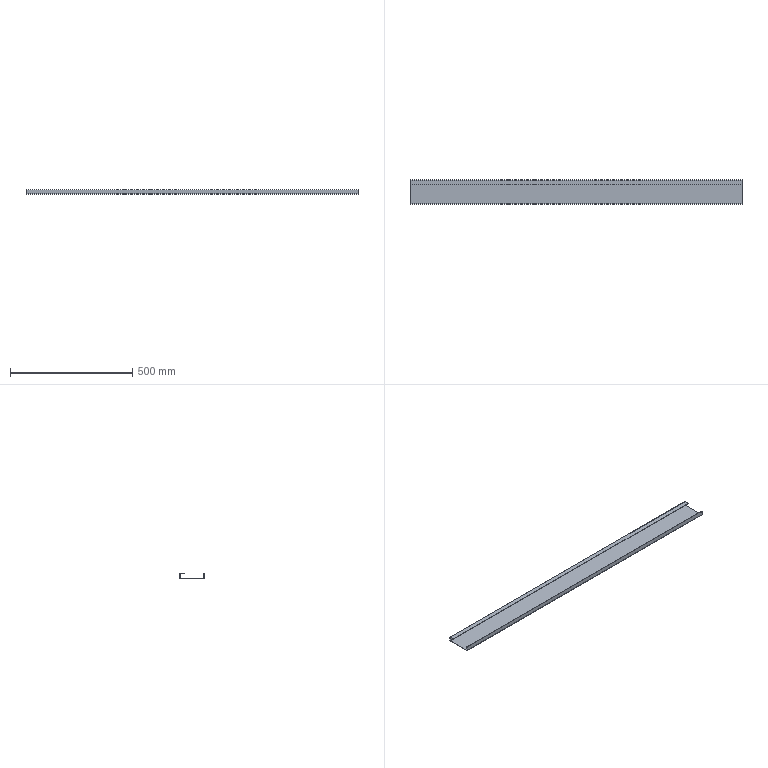Part | STEP file | 电柜护栏3踢脚Plate | 1 solid | 18 faces | box 1360 x 100 x 20 mm | volume 312623 mm3 | plane 12 | cylinder 6 | commonest cylinder face diameters 2 x3 5 x3
STEP:
#1=CARTESIAN_POINT('',(0.,0.,0.));
#2=DIRECTION('',(0.,0.,1.));
#3=DIRECTION('',(1.,0.,0.));
#4=AXIS2_PLACEMENT_3D('',#1,#2,#3);
#5=CARTESIAN_POINT('',(-680.,1.5,2.5));
#6=VERTEX_POINT('',#5);
#7=CARTESIAN_POINT('',(-680.,1.5,20.));
#8=VERTEX_POINT('',#7);
#9=CARTESIAN_POINT('',(-680.,1.5,2.5));
#10=DIRECTION('',(0.,0.,1.));
#11=VECTOR('',#10,1.);
#12=LINE('',#9,#11);
#13=CARTESIAN_POINT('',(680.,1.5,2.5));
#14=DIRECTION('',(0.,-1.,0.));
#15=DIRECTION('',(0.,0.,-1.));
#16=AXIS2_PLACEMENT_3D('',#13,#14,#15);
#17=PLANE('',#16);
#18=CARTESIAN_POINT('',(0.,-1360.));
#19=DIRECTION('',(-1.,0.));
#20=VECTOR('',#19,1.);
#21=LINE('',#18,#20);
#22=(GEOMETRIC_REPRESENTATION_CONTEXT(2)PARAMETRIC_REPRESENTATION_CONTEXT()REPRESENTATION_CONTEXT('',''));
#23=DEFINITIONAL_REPRESENTATION('',(#21),#22);
#24=PCURVE('',#17,#23);
#25=CARTESIAN_POINT('',(-680.,2.5,2.5));
#26=DIRECTION('',(-1.,0.,0.));
#27=DIRECTION('',(0.,0.,1.));
#28=AXIS2_PLACEMENT_3D('',#25,#26,#27);
#29=PLANE('',#28);
#30=CARTESIAN_POINT('',(0.,-1.));
#31=DIRECTION('',(1.,0.));
#32=VECTOR('',#31,1.);
#33=LINE('',#30,#32);
#34=(GEOMETRIC_REPRESENTATION_CONTEXT(2)PARAMETRIC_REPRESENTATION_CONTEXT()REPRESENTATION_CONTEXT('',''));
#35=DEFINITIONAL_REPRESENTATION('',(#33),#34);
#36=PCURVE('',#29,#35);
#37=SURFACE_CURVE('',#12,(#24,#36),.PCURVE_S1.);
#38=EDGE_CURVE('',#6,#8,#37,.T.);
#39=ORIENTED_EDGE('',*,*,#38,.T.);
#40=CARTESIAN_POINT('',(680.,1.5,20.));
#41=VERTEX_POINT('',#40);
#42=CARTESIAN_POINT('',(680.,1.5,20.));
#43=DIRECTION('',(-1.,0.,0.));
#44=VECTOR('',#43,1.);
#45=LINE('',#42,#44);
#46=CARTESIAN_POINT('',(-17.5,0.));
#47=DIRECTION('',(0.,-1.));
#48=VECTOR('',#47,1.);
#49=LINE('',#46,#48);
#50=(GEOMETRIC_REPRESENTATION_CONTEXT(2)PARAMETRIC_REPRESENTATION_CONTEXT()REPRESENTATION_CONTEXT('',''));
#51=DEFINITIONAL_REPRESENTATION('',(#49),#50);
#52=PCURVE('',#17,#51);
#53=CARTESIAN_POINT('',(680.,0.,20.));
#54=DIRECTION('',(0.,0.,1.));
#55=DIRECTION('',(1.,0.,0.));
#56=AXIS2_PLACEMENT_3D('',#53,#54,#55);
#57=PLANE('',#56);
#58=CARTESIAN_POINT('',(0.,1.5));
#59=DIRECTION('',(-1.,0.));
#60=VECTOR('',#59,1.);
#61=LINE('',#58,#60);
#62=(GEOMETRIC_REPRESENTATION_CONTEXT(2)PARAMETRIC_REPRESENTATION_CONTEXT()REPRESENTATION_CONTEXT('',''));
#63=DEFINITIONAL_REPRESENTATION('',(#61),#62);
#64=PCURVE('',#57,#63);
#65=SURFACE_CURVE('',#45,(#52,#64),.PCURVE_S1.);
#66=EDGE_CURVE('',#41,#8,#65,.T.);
#67=ORIENTED_EDGE('',*,*,#66,.F.);
#68=CARTESIAN_POINT('',(680.,1.5,2.5));
#69=VERTEX_POINT('',#68);
#70=CARTESIAN_POINT('',(680.,1.5,2.5));
#71=DIRECTION('',(0.,0.,1.));
#72=VECTOR('',#71,1.);
#73=LINE('',#70,#72);
#74=CARTESIAN_POINT('',(0.,0.));
#75=DIRECTION('',(-1.,0.));
#76=VECTOR('',#75,1.);
#77=LINE('',#74,#76);
#78=(GEOMETRIC_REPRESENTATION_CONTEXT(2)PARAMETRIC_REPRESENTATION_CONTEXT()REPRESENTATION_CONTEXT('',''));
#79=DEFINITIONAL_REPRESENTATION('',(#77),#78);
#80=PCURVE('',#17,#79);
#81=CARTESIAN_POINT('',(680.,2.5,2.5));
#82=DIRECTION('',(-1.,0.,0.));
#83=DIRECTION('',(0.,0.,1.));
#84=AXIS2_PLACEMENT_3D('',#81,#82,#83);
#85=PLANE('',#84);
#86=CARTESIAN_POINT('',(0.,-1.));
#87=DIRECTION('',(1.,0.));
#88=VECTOR('',#87,1.);
#89=LINE('',#86,#88);
#90=(GEOMETRIC_REPRESENTATION_CONTEXT(2)PARAMETRIC_REPRESENTATION_CONTEXT()REPRESENTATION_CONTEXT('',''));
#91=DEFINITIONAL_REPRESENTATION('',(#89),#90);
#92=PCURVE('',#85,#91);
#93=SURFACE_CURVE('',#73,(#80,#92),.PCURVE_S1.);
#94=EDGE_CURVE('',#69,#41,#93,.T.);
#95=ORIENTED_EDGE('',*,*,#94,.F.);
#96=CARTESIAN_POINT('',(680.,1.5,2.5));
#97=DIRECTION('',(-1.,0.,0.));
#98=VECTOR('',#97,1.);
#99=LINE('',#96,#98);
#100=CARTESIAN_POINT('',(0.,0.));
#101=DIRECTION('',(0.,-1.));
#102=VECTOR('',#101,1.);
#103=LINE('',#100,#102);
#104=(GEOMETRIC_REPRESENTATION_CONTEXT(2)PARAMETRIC_REPRESENTATION_CONTEXT()REPRESENTATION_CONTEXT('',''));
#105=DEFINITIONAL_REPRESENTATION('',(#103),#104);
#106=PCURVE('',#17,#105);
#107=CARTESIAN_POINT('',(680.,2.5,2.5));
#108=DIRECTION('',(-1.,0.,0.));
#109=DIRECTION('',(0.,0.,1.));
#110=AXIS2_PLACEMENT_3D('',#107,#108,#109);
#111=CYLINDRICAL_SURFACE('',#110,1.);
#112=CARTESIAN_POINT('',(4.712,0.));
#113=DIRECTION('',(0.,1.));
#114=VECTOR('',#113,1.);
#115=LINE('',#112,#114);
#116=(GEOMETRIC_REPRESENTATION_CONTEXT(2)PARAMETRIC_REPRESENTATION_CONTEXT()REPRESENTATION_CONTEXT('',''));
#117=DEFINITIONAL_REPRESENTATION('',(#115),#116);
#118=PCURVE('',#111,#117);
#119=SURFACE_CURVE('',#99,(#106,#118),.PCURVE_S1.);
#120=EDGE_CURVE('',#69,#6,#119,.T.);
#121=ORIENTED_EDGE('',*,*,#120,.T.);
#122=EDGE_LOOP('',(#39,#67,#95,#121));
#123=FACE_BOUND('',#122,.T.);
#124=ADVANCED_FACE('',(#123),#17,.F.);
#125=CARTESIAN_POINT('',(-680.,0.,20.));
#126=VERTEX_POINT('',#125);
#127=CARTESIAN_POINT('',(-680.,0.,20.));
#128=DIRECTION('',(0.,1.,0.));
#129=VECTOR('',#128,1.);
#130=LINE('',#127,#129);
#131=CARTESIAN_POINT('',(-1360.,0.));
#132=DIRECTION('',(0.,1.));
#133=VECTOR('',#132,1.);
#134=LINE('',#131,#133);
#135=(GEOMETRIC_REPRESENTATION_CONTEXT(2)PARAMETRIC_REPRESENTATION_CONTEXT()REPRESENTATION_CONTEXT('',''));
#136=DEFINITIONAL_REPRESENTATION('',(#134),#135);
#137=PCURVE('',#57,#136);
#138=CARTESIAN_POINT('',(17.5,-2.5));
#139=DIRECTION('',(0.,1.));
#140=VECTOR('',#139,1.);
#141=LINE('',#138,#140);
#142=(GEOMETRIC_REPRESENTATION_CONTEXT(2)PARAMETRIC_REPRESENTATION_CONTEXT()REPRESENTATION_CONTEXT('',''));
#143=DEFINITIONAL_REPRESENTATION('',(#141),#142);
#144=PCURVE('',#29,#143);
#145=SURFACE_CURVE('',#130,(#137,#144),.PCURVE_S1.);
#146=EDGE_CURVE('',#126,#8,#145,.T.);
#147=ORIENTED_EDGE('',*,*,#146,.F.);
#148=CARTESIAN_POINT('',(680.,0.,20.));
#149=VERTEX_POINT('',#148);
#150=CARTESIAN_POINT('',(680.,0.,20.));
#151=DIRECTION('',(-1.,0.,0.));
#152=VECTOR('',#151,1.);
#153=LINE('',#150,#152);
#154=CARTESIAN_POINT('',(0.,0.));
#155=DIRECTION('',(-1.,0.));
#156=VECTOR('',#155,1.);
#157=LINE('',#154,#156);
#158=(GEOMETRIC_REPRESENTATION_CONTEXT(2)PARAMETRIC_REPRESENTATION_CONTEXT()REPRESENTATION_CONTEXT('',''));
#159=DEFINITIONAL_REPRESENTATION('',(#157),#158);
#160=PCURVE('',#57,#159);
#161=CARTESIAN_POINT('',(680.,0.,2.5));
#162=DIRECTION('',(0.,-1.,0.));
#163=DIRECTION('',(0.,0.,-1.));
#164=AXIS2_PLACEMENT_3D('',#161,#162,#163);
#165=PLANE('',#164);
#166=CARTESIAN_POINT('',(-17.5,0.));
#167=DIRECTION('',(0.,-1.));
#168=VECTOR('',#167,1.);
#169=LINE('',#166,#168);
#170=(GEOMETRIC_REPRESENTATION_CONTEXT(2)PARAMETRIC_REPRESENTATION_CONTEXT()REPRESENTATION_CONTEXT('',''));
#171=DEFINITIONAL_REPRESENTATION('',(#169),#170);
#172=PCURVE('',#165,#171);
#173=SURFACE_CURVE('',#153,(#160,#172),.PCURVE_S1.);
#174=EDGE_CURVE('',#149,#126,#173,.T.);
#175=ORIENTED_EDGE('',*,*,#174,.F.);
#176=CARTESIAN_POINT('',(680.,0.,20.));
#177=DIRECTION('',(0.,1.,0.));
#178=VECTOR('',#177,1.);
#179=LINE('',#176,#178);
#180=CARTESIAN_POINT('',(0.,0.));
#181=DIRECTION('',(0.,1.));
#182=VECTOR('',#181,1.);
#183=LINE('',#180,#182);
#184=(GEOMETRIC_REPRESENTATION_CONTEXT(2)PARAMETRIC_REPRESENTATION_CONTEXT()REPRESENTATION_CONTEXT('',''));
#185=DEFINITIONAL_REPRESENTATION('',(#183),#184);
#186=PCURVE('',#57,#185);
#187=CARTESIAN_POINT('',(17.5,-2.5));
#188=DIRECTION('',(0.,1.));
#189=VECTOR('',#188,1.);
#190=LINE('',#187,#189);
#191=(GEOMETRIC_REPRESENTATION_CONTEXT(2)PARAMETRIC_REPRESENTATION_CONTEXT()REPRESENTATION_CONTEXT('',''));
#192=DEFINITIONAL_REPRESENTATION('',(#190),#191);
#193=PCURVE('',#85,#192);
#194=SURFACE_CURVE('',#179,(#186,#193),.PCURVE_S1.);
#195=EDGE_CURVE('',#149,#41,#194,.T.);
#196=ORIENTED_EDGE('',*,*,#195,.T.);
#197=ORIENTED_EDGE('',*,*,#66,.T.);
#198=EDGE_LOOP('',(#147,#175,#196,#197));
#199=FACE_BOUND('',#198,.T.);
#200=ADVANCED_FACE('',(#199),#57,.T.);
#201=CARTESIAN_POINT('',(-680.,0.,2.5));
#202=VERTEX_POINT('',#201);
#203=CARTESIAN_POINT('',(-680.,0.,2.5));
#204=DIRECTION('',(0.,0.,1.));
#205=VECTOR('',#204,1.);
#206=LINE('',#203,#205);
#207=CARTESIAN_POINT('',(0.,-1360.));
#208=DIRECTION('',(-1.,0.));
#209=VECTOR('',#208,1.);
#210=LINE('',#207,#209);
#211=(GEOMETRIC_REPRESENTATION_CONTEXT(2)PARAMETRIC_REPRESENTATION_CONTEXT()REPRESENTATION_CONTEXT('',''));
#212=DEFINITIONAL_REPRESENTATION('',(#210),#211);
#213=PCURVE('',#165,#212);
#214=CARTESIAN_POINT('',(0.,-2.5));
#215=DIRECTION('',(1.,0.));
#216=VECTOR('',#215,1.);
#217=LINE('',#214,#216);
#218=(GEOMETRIC_REPRESENTATION_CONTEXT(2)PARAMETRIC_REPRESENTATION_CONTEXT()REPRESENTATION_CONTEXT('',''));
#219=DEFINITIONAL_REPRESENTATION('',(#217),#218);
#220=PCURVE('',#29,#219);
#221=SURFACE_CURVE('',#206,(#213,#220),.PCURVE_S1.);
#222=EDGE_CURVE('',#202,#126,#221,.T.);
#223=ORIENTED_EDGE('',*,*,#222,.F.);
#224=CARTESIAN_POINT('',(680.,0.,2.5));
#225=VERTEX_POINT('',#224);
#226=CARTESIAN_POINT('',(680.,0.,2.5));
#227=DIRECTION('',(-1.,0.,0.));
#228=VECTOR('',#227,1.);
#229=LINE('',#226,#228);
#230=CARTESIAN_POINT('',(0.,0.));
#231=DIRECTION('',(0.,-1.));
#232=VECTOR('',#231,1.);
#233=LINE('',#230,#232);
#234=(GEOMETRIC_REPRESENTATION_CONTEXT(2)PARAMETRIC_REPRESENTATION_CONTEXT()REPRESENTATION_CONTEXT('',''));
#235=DEFINITIONAL_REPRESENTATION('',(#233),#234);
#236=PCURVE('',#165,#235);
#237=CARTESIAN_POINT('',(680.,2.5,2.5));
#238=DIRECTION('',(-1.,0.,0.));
#239=DIRECTION('',(0.,0.,1.));
#240=AXIS2_PLACEMENT_3D('',#237,#238,#239);
#241=CYLINDRICAL_SURFACE('',#240,2.5);
#242=CARTESIAN_POINT('',(4.712,0.));
#243=DIRECTION('',(0.,1.));
#244=VECTOR('',#243,1.);
#245=LINE('',#242,#244);
#246=(GEOMETRIC_REPRESENTATION_CONTEXT(2)PARAMETRIC_REPRESENTATION_CONTEXT()REPRESENTATION_CONTEXT('',''));
#247=DEFINITIONAL_REPRESENTATION('',(#245),#246);
#248=PCURVE('',#241,#247);
#249=SURFACE_CURVE('',#229,(#236,#248),.PCURVE_S1.);
#250=EDGE_CURVE('',#225,#202,#249,.T.);
#251=ORIENTED_EDGE('',*,*,#250,.F.);
#252=CARTESIAN_POINT('',(680.,0.,2.5));
#253=DIRECTION('',(0.,0.,1.));
#254=VECTOR('',#253,1.);
#255=LINE('',#252,#254);
#256=CARTESIAN_POINT('',(0.,0.));
#257=DIRECTION('',(-1.,0.));
#258=VECTOR('',#257,1.);
#259=LINE('',#256,#258);
#260=(GEOMETRIC_REPRESENTATION_CONTEXT(2)PARAMETRIC_REPRESENTATION_CONTEXT()REPRESENTATION_CONTEXT('',''));
#261=DEFINITIONAL_REPRESENTATION('',(#259),#260);
#262=PCURVE('',#165,#261);
#263=CARTESIAN_POINT('',(0.,-2.5));
#264=DIRECTION('',(1.,0.));
#265=VECTOR('',#264,1.);
#266=LINE('',#263,#265);
#267=(GEOMETRIC_REPRESENTATION_CONTEXT(2)PARAMETRIC_REPRESENTATION_CONTEXT()REPRESENTATION_CONTEXT('',''));
#268=DEFINITIONAL_REPRESENTATION('',(#266),#267);
#269=PCURVE('',#85,#268);
#270=SURFACE_CURVE('',#255,(#262,#269),.PCURVE_S1.);
#271=EDGE_CURVE('',#225,#149,#270,.T.);
#272=ORIENTED_EDGE('',*,*,#271,.T.);
#273=ORIENTED_EDGE('',*,*,#174,.T.);
#274=EDGE_LOOP('',(#223,#251,#272,#273));
#275=FACE_BOUND('',#274,.T.);
#276=ADVANCED_FACE('',(#275),#165,.T.);
#277=CARTESIAN_POINT('',(-680.,2.5,0.));
#278=VERTEX_POINT('',#277);
#279=CARTESIAN_POINT('',(-680.,2.5,2.5));
#280=DIRECTION('',(-1.,0.,0.));
#281=DIRECTION('',(0.,0.,1.));
#282=AXIS2_PLACEMENT_3D('',#279,#280,#281);
#283=CIRCLE('',#282,2.5);
#284=CARTESIAN_POINT('',(0.,1360.));
#285=DIRECTION('',(1.,0.));
#286=VECTOR('',#285,1.);
#287=LINE('',#284,#286);
#288=(GEOMETRIC_REPRESENTATION_CONTEXT(2)PARAMETRIC_REPRESENTATION_CONTEXT()REPRESENTATION_CONTEXT('',''));
#289=DEFINITIONAL_REPRESENTATION('',(#287),#288);
#290=PCURVE('',#241,#289);
#291=CARTESIAN_POINT('',(0.,0.));
#292=DIRECTION('',(1.,0.));
#293=AXIS2_PLACEMENT_2D('',#291,#292);
#294=CIRCLE('',#293,2.5);
#295=(GEOMETRIC_REPRESENTATION_CONTEXT(2)PARAMETRIC_REPRESENTATION_CONTEXT()REPRESENTATION_CONTEXT('',''));
#296=DEFINITIONAL_REPRESENTATION('',(#294),#295);
#297=PCURVE('',#29,#296);
#298=SURFACE_CURVE('',#283,(#290,#297),.PCURVE_S1.);
#299=EDGE_CURVE('',#278,#202,#298,.T.);
#300=ORIENTED_EDGE('',*,*,#299,.F.);
#301=CARTESIAN_POINT('',(680.,2.5,0.));
#302=VERTEX_POINT('',#301);
#303=CARTESIAN_POINT('',(680.,2.5,0.));
#304=DIRECTION('',(-1.,0.,0.));
#305=VECTOR('',#304,1.);
#306=LINE('',#303,#305);
#307=CARTESIAN_POINT('',(3.142,0.));
#308=DIRECTION('',(0.,1.));
#309=VECTOR('',#308,1.);
#310=LINE('',#307,#309);
#311=(GEOMETRIC_REPRESENTATION_CONTEXT(2)PARAMETRIC_REPRESENTATION_CONTEXT()REPRESENTATION_CONTEXT('',''));
#312=DEFINITIONAL_REPRESENTATION('',(#310),#311);
#313=PCURVE('',#241,#312);
#314=CARTESIAN_POINT('',(680.,2.5,0.));
#315=DIRECTION('',(0.,0.,-1.));
#316=DIRECTION('',(-1.,0.,0.));
#317=AXIS2_PLACEMENT_3D('',#314,#315,#316);
#318=PLANE('',#317);
#319=CARTESIAN_POINT('',(0.,0.));
#320=DIRECTION('',(1.,0.));
#321=VECTOR('',#320,1.);
#322=LINE('',#319,#321);
#323=(GEOMETRIC_REPRESENTATION_CONTEXT(2)PARAMETRIC_REPRESENTATION_CONTEXT()REPRESENTATION_CONTEXT('',''));
#324=DEFINITIONAL_REPRESENTATION('',(#322),#323);
#325=PCURVE('',#318,#324);
#326=SURFACE_CURVE('',#306,(#313,#325),.PCURVE_S1.);
#327=EDGE_CURVE('',#302,#278,#326,.T.);
#328=ORIENTED_EDGE('',*,*,#327,.F.);
#329=CARTESIAN_POINT('',(680.,2.5,2.5));
#330=DIRECTION('',(-1.,0.,0.));
#331=DIRECTION('',(0.,0.,1.));
#332=AXIS2_PLACEMENT_3D('',#329,#330,#331);
#333=CIRCLE('',#332,2.5);
#334=CARTESIAN_POINT('',(0.,0.));
#335=DIRECTION('',(1.,0.));
#336=VECTOR('',#335,1.);
#337=LINE('',#334,#336);
#338=(GEOMETRIC_REPRESENTATION_CONTEXT(2)PARAMETRIC_REPRESENTATION_CONTEXT()REPRESENTATION_CONTEXT('',''));
#339=DEFINITIONAL_REPRESENTATION('',(#337),#338);
#340=PCURVE('',#241,#339);
#341=CARTESIAN_POINT('',(0.,0.));
#342=DIRECTION('',(1.,0.));
#343=AXIS2_PLACEMENT_2D('',#341,#342);
#344=CIRCLE('',#343,2.5);
#345=(GEOMETRIC_REPRESENTATION_CONTEXT(2)PARAMETRIC_REPRESENTATION_CONTEXT()REPRESENTATION_CONTEXT('',''));
#346=DEFINITIONAL_REPRESENTATION('',(#344),#345);
#347=PCURVE('',#85,#346);
#348=SURFACE_CURVE('',#333,(#340,#347),.PCURVE_S1.);
#349=EDGE_CURVE('',#302,#225,#348,.T.);
#350=ORIENTED_EDGE('',*,*,#349,.T.);
#351=ORIENTED_EDGE('',*,*,#250,.T.);
#352=EDGE_LOOP('',(#300,#328,#350,#351));
#353=FACE_BOUND('',#352,.T.);
#354=ADVANCED_FACE('',(#353),#241,.T.);
#355=CARTESIAN_POINT('',(-680.,97.5,0.));
#356=VERTEX_POINT('',#355);
#357=CARTESIAN_POINT('',(-680.,2.5,0.));
#358=DIRECTION('',(0.,-1.,0.));
#359=VECTOR('',#358,1.);
#360=LINE('',#357,#359);
#361=CARTESIAN_POINT('',(1360.,0.));
#362=DIRECTION('',(0.,-1.));
#363=VECTOR('',#362,1.);
#364=LINE('',#361,#363);
#365=(GEOMETRIC_REPRESENTATION_CONTEXT(2)PARAMETRIC_REPRESENTATION_CONTEXT()REPRESENTATION_CONTEXT('',''));
#366=DEFINITIONAL_REPRESENTATION('',(#364),#365);
#367=PCURVE('',#318,#366);
#368=CARTESIAN_POINT('',(-2.5,0.));
#369=DIRECTION('',(0.,-1.));
#370=VECTOR('',#369,1.);
#371=LINE('',#368,#370);
#372=(GEOMETRIC_REPRESENTATION_CONTEXT(2)PARAMETRIC_REPRESENTATION_CONTEXT()REPRESENTATION_CONTEXT('',''));
#373=DEFINITIONAL_REPRESENTATION('',(#371),#372);
#374=PCURVE('',#29,#373);
#375=SURFACE_CURVE('',#360,(#367,#374),.PCURVE_S1.);
#376=EDGE_CURVE('',#356,#278,#375,.T.);
#377=ORIENTED_EDGE('',*,*,#376,.F.);
#378=CARTESIAN_POINT('',(680.,97.5,0.));
#379=VERTEX_POINT('',#378);
#380=CARTESIAN_POINT('',(680.,97.5,0.));
#381=DIRECTION('',(-1.,0.,0.));
#382=VECTOR('',#381,1.);
#383=LINE('',#380,#382);
#384=CARTESIAN_POINT('',(0.,95.));
#385=DIRECTION('',(1.,0.));
#386=VECTOR('',#385,1.);
#387=LINE('',#384,#386);
#388=(GEOMETRIC_REPRESENTATION_CONTEXT(2)PARAMETRIC_REPRESENTATION_CONTEXT()REPRESENTATION_CONTEXT('',''));
#389=DEFINITIONAL_REPRESENTATION('',(#387),#388);
#390=PCURVE('',#318,#389);
#391=CARTESIAN_POINT('',(680.,97.5,2.5));
#392=DIRECTION('',(-1.,0.,0.));
#393=DIRECTION('',(0.,0.,1.));
#394=AXIS2_PLACEMENT_3D('',#391,#392,#393);
#395=CYLINDRICAL_SURFACE('',#394,2.5);
#396=CARTESIAN_POINT('',(3.142,0.));
#397=DIRECTION('',(0.,1.));
#398=VECTOR('',#397,1.);
#399=LINE('',#396,#398);
#400=(GEOMETRIC_REPRESENTATION_CONTEXT(2)PARAMETRIC_REPRESENTATION_CONTEXT()REPRESENTATION_CONTEXT('',''));
#401=DEFINITIONAL_REPRESENTATION('',(#399),#400);
#402=PCURVE('',#395,#401);
#403=SURFACE_CURVE('',#383,(#390,#402),.PCURVE_S1.);
#404=EDGE_CURVE('',#379,#356,#403,.T.);
#405=ORIENTED_EDGE('',*,*,#404,.F.);
#406=CARTESIAN_POINT('',(680.,2.5,0.));
#407=DIRECTION('',(0.,-1.,0.));
#408=VECTOR('',#407,1.);
#409=LINE('',#406,#408);
#410=CARTESIAN_POINT('',(0.,0.));
#411=DIRECTION('',(0.,-1.));
#412=VECTOR('',#411,1.);
#413=LINE('',#410,#412);
#414=(GEOMETRIC_REPRESENTATION_CONTEXT(2)PARAMETRIC_REPRESENTATION_CONTEXT()REPRESENTATION_CONTEXT('',''));
#415=DEFINITIONAL_REPRESENTATION('',(#413),#414);
#416=PCURVE('',#318,#415);
#417=CARTESIAN_POINT('',(-2.5,0.));
#418=DIRECTION('',(0.,-1.));
#419=VECTOR('',#418,1.);
#420=LINE('',#417,#419);
#421=(GEOMETRIC_REPRESENTATION_CONTEXT(2)PARAMETRIC_REPRESENTATION_CONTEXT()REPRESENTATION_CONTEXT('',''));
#422=DEFINITIONAL_REPRESENTATION('',(#420),#421);
#423=PCURVE('',#85,#422);
#424=SURFACE_CURVE('',#409,(#416,#423),.PCURVE_S1.);
#425=EDGE_CURVE('',#379,#302,#424,.T.);
#426=ORIENTED_EDGE('',*,*,#425,.T.);
#427=ORIENTED_EDGE('',*,*,#327,.T.);
#428=EDGE_LOOP('',(#377,#405,#426,#427));
#429=FACE_BOUND('',#428,.T.);
#430=ADVANCED_FACE('',(#429),#318,.T.);
#431=CARTESIAN_POINT('',(-680.,100.,2.5));
#432=VERTEX_POINT('',#431);
#433=CARTESIAN_POINT('',(-680.,97.5,2.5));
#434=DIRECTION('',(-1.,0.,0.));
#435=DIRECTION('',(0.,0.,-1.));
#436=AXIS2_PLACEMENT_3D('',#433,#434,#435);
#437=CIRCLE('',#436,2.5);
#438=CARTESIAN_POINT('',(-3.142,1360.));
#439=DIRECTION('',(1.,0.));
#440=VECTOR('',#439,1.);
#441=LINE('',#438,#440);
#442=(GEOMETRIC_REPRESENTATION_CONTEXT(2)PARAMETRIC_REPRESENTATION_CONTEXT()REPRESENTATION_CONTEXT('',''));
#443=DEFINITIONAL_REPRESENTATION('',(#441),#442);
#444=PCURVE('',#395,#443);
#445=CARTESIAN_POINT('',(0.,95.));
#446=DIRECTION('',(-1.,0.));
#447=AXIS2_PLACEMENT_2D('',#445,#446);
#448=CIRCLE('',#447,2.5);
#449=(GEOMETRIC_REPRESENTATION_CONTEXT(2)PARAMETRIC_REPRESENTATION_CONTEXT()REPRESENTATION_CONTEXT('',''));
#450=DEFINITIONAL_REPRESENTATION('',(#448),#449);
#451=PCURVE('',#29,#450);
#452=SURFACE_CURVE('',#437,(#444,#451),.PCURVE_S1.);
#453=EDGE_CURVE('',#432,#356,#452,.T.);
#454=ORIENTED_EDGE('',*,*,#453,.F.);
#455=CARTESIAN_POINT('',(680.,100.,2.5));
#456=VERTEX_POINT('',#455);
#457=CARTESIAN_POINT('',(680.,100.,2.5));
#458=DIRECTION('',(-1.,0.,0.));
#459=VECTOR('',#458,1.);
#460=LINE('',#457,#459);
#461=CARTESIAN_POINT('',(1.571,0.));
#462=DIRECTION('',(0.,1.));
#463=VECTOR('',#462,1.);
#464=LINE('',#461,#463);
#465=(GEOMETRIC_REPRESENTATION_CONTEXT(2)PARAMETRIC_REPRESENTATION_CONTEXT()REPRESENTATION_CONTEXT('',''));
#466=DEFINITIONAL_REPRESENTATION('',(#464),#465);
#467=PCURVE('',#395,#466);
#468=CARTESIAN_POINT('',(680.,100.,2.5));
#469=DIRECTION('',(0.,1.,0.));
#470=DIRECTION('',(0.,0.,1.));
#471=AXIS2_PLACEMENT_3D('',#468,#469,#470);
#472=PLANE('',#471);
#473=CARTESIAN_POINT('',(0.,0.));
#474=DIRECTION('',(0.,-1.));
#475=VECTOR('',#474,1.);
#476=LINE('',#473,#475);
#477=(GEOMETRIC_REPRESENTATION_CONTEXT(2)PARAMETRIC_REPRESENTATION_CONTEXT()REPRESENTATION_CONTEXT('',''));
#478=DEFINITIONAL_REPRESENTATION('',(#476),#477);
#479=PCURVE('',#472,#478);
#480=SURFACE_CURVE('',#460,(#467,#479),.PCURVE_S1.);
#481=EDGE_CURVE('',#456,#432,#480,.T.);
#482=ORIENTED_EDGE('',*,*,#481,.F.);
#483=CARTESIAN_POINT('',(680.,97.5,2.5));
#484=DIRECTION('',(-1.,0.,0.));
#485=DIRECTION('',(0.,0.,-1.));
#486=AXIS2_PLACEMENT_3D('',#483,#484,#485);
#487=CIRCLE('',#486,2.5);
#488=CARTESIAN_POINT('',(-3.142,0.));
#489=DIRECTION('',(1.,0.));
#490=VECTOR('',#489,1.);
#491=LINE('',#488,#490);
#492=(GEOMETRIC_REPRESENTATION_CONTEXT(2)PARAMETRIC_REPRESENTATION_CONTEXT()REPRESENTATION_CONTEXT('',''));
#493=DEFINITIONAL_REPRESENTATION('',(#491),#492);
#494=PCURVE('',#395,#493);
#495=CARTESIAN_POINT('',(0.,95.));
#496=DIRECTION('',(-1.,0.));
#497=AXIS2_PLACEMENT_2D('',#495,#496);
#498=CIRCLE('',#497,2.5);
#499=(GEOMETRIC_REPRESENTATION_CONTEXT(2)PARAMETRIC_REPRESENTATION_CONTEXT()REPRESENTATION_CONTEXT('',''));
#500=DEFINITIONAL_REPRESENTATION('',(#498),#499);
#501=PCURVE('',#85,#500);
#502=SURFACE_CURVE('',#487,(#494,#501),.PCURVE_S1.);
#503=EDGE_CURVE('',#456,#379,#502,.T.);
#504=ORIENTED_EDGE('',*,*,#503,.T.);
#505=ORIENTED_EDGE('',*,*,#404,.T.);
#506=EDGE_LOOP('',(#454,#482,#504,#505));
#507=FACE_BOUND('',#506,.T.);
#508=ADVANCED_FACE('',(#507),#395,.T.);
#509=CARTESIAN_POINT('',(-680.,100.,17.5));
#510=VERTEX_POINT('',#509);
#511=CARTESIAN_POINT('',(-680.,100.,2.5));
#512=DIRECTION('',(0.,0.,-1.));
#513=VECTOR('',#512,1.);
#514=LINE('',#511,#513);
#515=CARTESIAN_POINT('',(0.,-1360.));
#516=DIRECTION('',(-1.,0.));
#517=VECTOR('',#516,1.);
#518=LINE('',#515,#517);
#519=(GEOMETRIC_REPRESENTATION_CONTEXT(2)PARAMETRIC_REPRESENTATION_CONTEXT()REPRESENTATION_CONTEXT('',''));
#520=DEFINITIONAL_REPRESENTATION('',(#518),#519);
#521=PCURVE('',#472,#520);
#522=CARTESIAN_POINT('',(0.,97.5));
#523=DIRECTION('',(-1.,0.));
#524=VECTOR('',#523,1.);
#525=LINE('',#522,#524);
#526=(GEOMETRIC_REPRESENTATION_CONTEXT(2)PARAMETRIC_REPRESENTATION_CONTEXT()REPRESENTATION_CONTEXT('',''));
#527=DEFINITIONAL_REPRESENTATION('',(#525),#526);
#528=PCURVE('',#29,#527);
#529=SURFACE_CURVE('',#514,(#521,#528),.PCURVE_S1.);
#530=EDGE_CURVE('',#510,#432,#529,.T.);
#531=ORIENTED_EDGE('',*,*,#530,.F.);
#532=CARTESIAN_POINT('',(680.,100.,17.5));
#533=VERTEX_POINT('',#532);
#534=CARTESIAN_POINT('',(680.,100.,17.5));
#535=DIRECTION('',(-1.,0.,0.));
#536=VECTOR('',#535,1.);
#537=LINE('',#534,#536);
#538=CARTESIAN_POINT('',(15.,0.));
#539=DIRECTION('',(0.,-1.));
#540=VECTOR('',#539,1.);
#541=LINE('',#538,#540);
#542=(GEOMETRIC_REPRESENTATION_CONTEXT(2)PARAMETRIC_REPRESENTATION_CONTEXT()REPRESENTATION_CONTEXT('',''));
#543=DEFINITIONAL_REPRESENTATION('',(#541),#542);
#544=PCURVE('',#472,#543);
#545=CARTESIAN_POINT('',(680.,97.5,17.5));
#546=DIRECTION('',(-1.,0.,0.));
#547=DIRECTION('',(0.,0.,1.));
#548=AXIS2_PLACEMENT_3D('',#545,#546,#547);
#549=CYLINDRICAL_SURFACE('',#548,2.5);
#550=CARTESIAN_POINT('',(1.571,0.));
#551=DIRECTION('',(0.,1.));
#552=VECTOR('',#551,1.);
#553=LINE('',#550,#552);
#554=(GEOMETRIC_REPRESENTATION_CONTEXT(2)PARAMETRIC_REPRESENTATION_CONTEXT()REPRESENTATION_CONTEXT('',''));
#555=DEFINITIONAL_REPRESENTATION('',(#553),#554);
#556=PCURVE('',#549,#555);
#557=SURFACE_CURVE('',#537,(#544,#556),.PCURVE_S1.);
#558=EDGE_CURVE('',#533,#510,#557,.T.);
#559=ORIENTED_EDGE('',*,*,#558,.F.);
#560=CARTESIAN_POINT('',(680.,100.,2.5));
#561=DIRECTION('',(0.,0.,-1.));
#562=VECTOR('',#561,1.);
#563=LINE('',#560,#562);
#564=CARTESIAN_POINT('',(0.,0.));
#565=DIRECTION('',(-1.,0.));
#566=VECTOR('',#565,1.);
#567=LINE('',#564,#566);
#568=(GEOMETRIC_REPRESENTATION_CONTEXT(2)PARAMETRIC_REPRESENTATION_CONTEXT()REPRESENTATION_CONTEXT('',''));
#569=DEFINITIONAL_REPRESENTATION('',(#567),#568);
#570=PCURVE('',#472,#569);
#571=CARTESIAN_POINT('',(0.,97.5));
#572=DIRECTION('',(-1.,0.));
#573=VECTOR('',#572,1.);
#574=LINE('',#571,#573);
#575=(GEOMETRIC_REPRESENTATION_CONTEXT(2)PARAMETRIC_REPRESENTATION_CONTEXT()REPRESENTATION_CONTEXT('',''));
#576=DEFINITIONAL_REPRESENTATION('',(#574),#575);
#577=PCURVE('',#85,#576);
#578=SURFACE_CURVE('',#563,(#570,#577),.PCURVE_S1.);
#579=EDGE_CURVE('',#533,#456,#578,.T.);
#580=ORIENTED_EDGE('',*,*,#579,.T.);
#581=ORIENTED_EDGE('',*,*,#481,.T.);
#582=EDGE_LOOP('',(#531,#559,#580,#581));
#583=FACE_BOUND('',#582,.T.);
#584=ADVANCED_FACE('',(#583),#472,.T.);
#585=CARTESIAN_POINT('',(-680.,97.5,20.));
#586=VERTEX_POINT('',#585);
#587=CARTESIAN_POINT('',(-680.,97.5,17.5));
#588=DIRECTION('',(-1.,0.,0.));
#589=DIRECTION('',(0.,0.,-1.));
#590=AXIS2_PLACEMENT_3D('',#587,#588,#589);
#591=CIRCLE('',#590,2.5);
#592=CARTESIAN_POINT('',(-3.142,1360.));
#593=DIRECTION('',(1.,0.));
#594=VECTOR('',#593,1.);
#595=LINE('',#592,#594);
#596=(GEOMETRIC_REPRESENTATION_CONTEXT(2)PARAMETRIC_REPRESENTATION_CONTEXT()REPRESENTATION_CONTEXT('',''));
#597=DEFINITIONAL_REPRESENTATION('',(#595),#596);
#598=PCURVE('',#549,#597);
#599=CARTESIAN_POINT('',(15.,95.));
#600=DIRECTION('',(-1.,0.));
#601=AXIS2_PLACEMENT_2D('',#599,#600);
#602=CIRCLE('',#601,2.5);
#603=(GEOMETRIC_REPRESENTATION_CONTEXT(2)PARAMETRIC_REPRESENTATION_CONTEXT()REPRESENTATION_CONTEXT('',''));
#604=DEFINITIONAL_REPRESENTATION('',(#602),#603);
#605=PCURVE('',#29,#604);
#606=SURFACE_CURVE('',#591,(#598,#605),.PCURVE_S1.);
#607=EDGE_CURVE('',#586,#510,#606,.T.);
#608=ORIENTED_EDGE('',*,*,#607,.F.);
#609=CARTESIAN_POINT('',(680.,97.5,20.));
#610=VERTEX_POINT('',#609);
#611=CARTESIAN_POINT('',(680.,97.5,20.));
#612=DIRECTION('',(-1.,0.,0.));
#613=VECTOR('',#612,1.);
#614=LINE('',#611,#613);
#615=CARTESIAN_POINT('',(0.,0.));
#616=DIRECTION('',(0.,1.));
#617=VECTOR('',#616,1.);
#618=LINE('',#615,#617);
#619=(GEOMETRIC_REPRESENTATION_CONTEXT(2)PARAMETRIC_REPRESENTATION_CONTEXT()REPRESENTATION_CONTEXT('',''));
#620=DEFINITIONAL_REPRESENTATION('',(#618),#619);
#621=PCURVE('',#549,#620);
#622=CARTESIAN_POINT('',(680.,97.5,20.));
#623=DIRECTION('',(0.,0.,1.));
#624=DIRECTION('',(1.,0.,0.));
#625=AXIS2_PLACEMENT_3D('',#622,#623,#624);
#626=PLANE('',#625);
#627=CARTESIAN_POINT('',(0.,0.));
#628=DIRECTION('',(-1.,0.));
#629=VECTOR('',#628,1.);
#630=LINE('',#627,#629);
#631=(GEOMETRIC_REPRESENTATION_CONTEXT(2)PARAMETRIC_REPRESENTATION_CONTEXT()REPRESENTATION_CONTEXT('',''));
#632=DEFINITIONAL_REPRESENTATION('',(#630),#631);
#633=PCURVE('',#626,#632);
#634=SURFACE_CURVE('',#614,(#621,#633),.PCURVE_S1.);
#635=EDGE_CURVE('',#610,#586,#634,.T.);
#636=ORIENTED_EDGE('',*,*,#635,.F.);
#637=CARTESIAN_POINT('',(680.,97.5,17.5));
#638=DIRECTION('',(-1.,0.,0.));
#639=DIRECTION('',(0.,0.,-1.));
#640=AXIS2_PLACEMENT_3D('',#637,#638,#639);
#641=CIRCLE('',#640,2.5);
#642=CARTESIAN_POINT('',(-3.142,0.));
#643=DIRECTION('',(1.,0.));
#644=VECTOR('',#643,1.);
#645=LINE('',#642,#644);
#646=(GEOMETRIC_REPRESENTATION_CONTEXT(2)PARAMETRIC_REPRESENTATION_CONTEXT()REPRESENTATION_CONTEXT('',''));
#647=DEFINITIONAL_REPRESENTATION('',(#645),#646);
#648=PCURVE('',#549,#647);
#649=CARTESIAN_POINT('',(15.,95.));
#650=DIRECTION('',(-1.,0.));
#651=AXIS2_PLACEMENT_2D('',#649,#650);
#652=CIRCLE('',#651,2.5);
#653=(GEOMETRIC_REPRESENTATION_CONTEXT(2)PARAMETRIC_REPRESENTATION_CONTEXT()REPRESENTATION_CONTEXT('',''));
#654=DEFINITIONAL_REPRESENTATION('',(#652),#653);
#655=PCURVE('',#85,#654);
#656=SURFACE_CURVE('',#641,(#648,#655),.PCURVE_S1.);
#657=EDGE_CURVE('',#610,#533,#656,.T.);
#658=ORIENTED_EDGE('',*,*,#657,.T.);
#659=ORIENTED_EDGE('',*,*,#558,.T.);
#660=EDGE_LOOP('',(#608,#636,#658,#659));
#661=FACE_BOUND('',#660,.T.);
#662=ADVANCED_FACE('',(#661),#549,.T.);
#663=CARTESIAN_POINT('',(-680.,80.,20.));
#664=VERTEX_POINT('',#663);
#665=CARTESIAN_POINT('',(-680.,97.5,20.));
#666=DIRECTION('',(0.,1.,0.));
#667=VECTOR('',#666,1.);
#668=LINE('',#665,#667);
#669=CARTESIAN_POINT('',(-1360.,0.));
#670=DIRECTION('',(0.,1.));
#671=VECTOR('',#670,1.);
#672=LINE('',#669,#671);
#673=(GEOMETRIC_REPRESENTATION_CONTEXT(2)PARAMETRIC_REPRESENTATION_CONTEXT()REPRESENTATION_CONTEXT('',''));
#674=DEFINITIONAL_REPRESENTATION('',(#672),#673);
#675=PCURVE('',#626,#674);
#676=CARTESIAN_POINT('',(17.5,95.));
#677=DIRECTION('',(0.,1.));
#678=VECTOR('',#677,1.);
#679=LINE('',#676,#678);
#680=(GEOMETRIC_REPRESENTATION_CONTEXT(2)PARAMETRIC_REPRESENTATION_CONTEXT()REPRESENTATION_CONTEXT('',''));
#681=DEFINITIONAL_REPRESENTATION('',(#679),#680);
#682=PCURVE('',#29,#681);
#683=SURFACE_CURVE('',#668,(#675,#682),.PCURVE_S1.);
#684=EDGE_CURVE('',#664,#586,#683,.T.);
#685=ORIENTED_EDGE('',*,*,#684,.F.);
#686=CARTESIAN_POINT('',(680.,80.,20.));
#687=VERTEX_POINT('',#686);
#688=CARTESIAN_POINT('',(680.,80.,20.));
#689=DIRECTION('',(-1.,0.,0.));
#690=VECTOR('',#689,1.);
#691=LINE('',#688,#690);
#692=CARTESIAN_POINT('',(0.,-17.5));
#693=DIRECTION('',(-1.,0.));
#694=VECTOR('',#693,1.);
#695=LINE('',#692,#694);
#696=(GEOMETRIC_REPRESENTATION_CONTEXT(2)PARAMETRIC_REPRESENTATION_CONTEXT()REPRESENTATION_CONTEXT('',''));
#697=DEFINITIONAL_REPRESENTATION('',(#695),#696);
#698=PCURVE('',#626,#697);
#699=CARTESIAN_POINT('',(680.,80.,18.5));
#700=DIRECTION('',(0.,-1.,0.));
#701=DIRECTION('',(0.,0.,-1.));
#702=AXIS2_PLACEMENT_3D('',#699,#700,#701);
#703=PLANE('',#702);
#704=CARTESIAN_POINT('',(-1.5,0.));
#705=DIRECTION('',(0.,-1.));
#706=VECTOR('',#705,1.);
#707=LINE('',#704,#706);
#708=(GEOMETRIC_REPRESENTATION_CONTEXT(2)PARAMETRIC_REPRESENTATION_CONTEXT()REPRESENTATION_CONTEXT('',''));
#709=DEFINITIONAL_REPRESENTATION('',(#707),#708);
#710=PCURVE('',#703,#709);
#711=SURFACE_CURVE('',#691,(#698,#710),.PCURVE_S1.);
#712=EDGE_CURVE('',#687,#664,#711,.T.);
#713=ORIENTED_EDGE('',*,*,#712,.F.);
#714=CARTESIAN_POINT('',(680.,97.5,20.));
#715=DIRECTION('',(0.,1.,0.));
#716=VECTOR('',#715,1.);
#717=LINE('',#714,#716);
#718=CARTESIAN_POINT('',(0.,0.));
#719=DIRECTION('',(0.,1.));
#720=VECTOR('',#719,1.);
#721=LINE('',#718,#720);
#722=(GEOMETRIC_REPRESENTATION_CONTEXT(2)PARAMETRIC_REPRESENTATION_CONTEXT()REPRESENTATION_CONTEXT('',''));
#723=DEFINITIONAL_REPRESENTATION('',(#721),#722);
#724=PCURVE('',#626,#723);
#725=CARTESIAN_POINT('',(17.5,95.));
#726=DIRECTION('',(0.,1.));
#727=VECTOR('',#726,1.);
#728=LINE('',#725,#727);
#729=(GEOMETRIC_REPRESENTATION_CONTEXT(2)PARAMETRIC_REPRESENTATION_CONTEXT()REPRESENTATION_CONTEXT('',''));
#730=DEFINITIONAL_REPRESENTATION('',(#728),#729);
#731=PCURVE('',#85,#730);
#732=SURFACE_CURVE('',#717,(#724,#731),.PCURVE_S1.);
#733=EDGE_CURVE('',#687,#610,#732,.T.);
#734=ORIENTED_EDGE('',*,*,#733,.T.);
#735=ORIENTED_EDGE('',*,*,#635,.T.);
#736=EDGE_LOOP('',(#685,#713,#734,#735));
#737=FACE_BOUND('',#736,.T.);
#738=ADVANCED_FACE('',(#737),#626,.T.);
#739=CARTESIAN_POINT('',(-680.,80.,18.5));
#740=VERTEX_POINT('',#739);
#741=CARTESIAN_POINT('',(-680.,80.,18.5));
#742=DIRECTION('',(0.,0.,1.));
#743=VECTOR('',#742,1.);
#744=LINE('',#741,#743);
#745=CARTESIAN_POINT('',(0.,-1360.));
#746=DIRECTION('',(-1.,0.));
#747=VECTOR('',#746,1.);
#748=LINE('',#745,#747);
#749=(GEOMETRIC_REPRESENTATION_CONTEXT(2)PARAMETRIC_REPRESENTATION_CONTEXT()REPRESENTATION_CONTEXT('',''));
#750=DEFINITIONAL_REPRESENTATION('',(#748),#749);
#751=PCURVE('',#703,#750);
#752=CARTESIAN_POINT('',(16.,77.5));
#753=DIRECTION('',(1.,0.));
#754=VECTOR('',#753,1.);
#755=LINE('',#752,#754);
#756=(GEOMETRIC_REPRESENTATION_CONTEXT(2)PARAMETRIC_REPRESENTATION_CONTEXT()REPRESENTATION_CONTEXT('',''));
#757=DEFINITIONAL_REPRESENTATION('',(#755),#756);
#758=PCURVE('',#29,#757);
#759=SURFACE_CURVE('',#744,(#751,#758),.PCURVE_S1.);
#760=EDGE_CURVE('',#740,#664,#759,.T.);
#761=ORIENTED_EDGE('',*,*,#760,.F.);
#762=CARTESIAN_POINT('',(680.,80.,18.5));
#763=VERTEX_POINT('',#762);
#764=CARTESIAN_POINT('',(680.,80.,18.5));
#765=DIRECTION('',(-1.,0.,0.));
#766=VECTOR('',#765,1.);
#767=LINE('',#764,#766);
#768=CARTESIAN_POINT('',(0.,0.));
#769=DIRECTION('',(0.,-1.));
#770=VECTOR('',#769,1.);
#771=LINE('',#768,#770);
#772=(GEOMETRIC_REPRESENTATION_CONTEXT(2)PARAMETRIC_REPRESENTATION_CONTEXT()REPRESENTATION_CONTEXT('',''));
#773=DEFINITIONAL_REPRESENTATION('',(#771),#772);
#774=PCURVE('',#703,#773);
#775=CARTESIAN_POINT('',(680.,97.5,18.5));
#776=DIRECTION('',(0.,0.,1.));
#777=DIRECTION('',(1.,0.,0.));
#778=AXIS2_PLACEMENT_3D('',#775,#776,#777);
#779=PLANE('',#778);
#780=CARTESIAN_POINT('',(0.,-17.5));
#781=DIRECTION('',(-1.,0.));
#782=VECTOR('',#781,1.);
#783=LINE('',#780,#782);
#784=(GEOMETRIC_REPRESENTATION_CONTEXT(2)PARAMETRIC_REPRESENTATION_CONTEXT()REPRESENTATION_CONTEXT('',''));
#785=DEFINITIONAL_REPRESENTATION('',(#783),#784);
#786=PCURVE('',#779,#785);
#787=SURFACE_CURVE('',#767,(#774,#786),.PCURVE_S1.);
#788=EDGE_CURVE('',#763,#740,#787,.T.);
#789=ORIENTED_EDGE('',*,*,#788,.F.);
#790=CARTESIAN_POINT('',(680.,80.,18.5));
#791=DIRECTION('',(0.,0.,1.));
#792=VECTOR('',#791,1.);
#793=LINE('',#790,#792);
#794=CARTESIAN_POINT('',(0.,0.));
#795=DIRECTION('',(-1.,0.));
#796=VECTOR('',#795,1.);
#797=LINE('',#794,#796);
#798=(GEOMETRIC_REPRESENTATION_CONTEXT(2)PARAMETRIC_REPRESENTATION_CONTEXT()REPRESENTATION_CONTEXT('',''));
#799=DEFINITIONAL_REPRESENTATION('',(#797),#798);
#800=PCURVE('',#703,#799);
#801=CARTESIAN_POINT('',(16.,77.5));
#802=DIRECTION('',(1.,0.));
#803=VECTOR('',#802,1.);
#804=LINE('',#801,#803);
#805=(GEOMETRIC_REPRESENTATION_CONTEXT(2)PARAMETRIC_REPRESENTATION_CONTEXT()REPRESENTATION_CONTEXT('',''));
#806=DEFINITIONAL_REPRESENTATION('',(#804),#805);
#807=PCURVE('',#85,#806);
#808=SURFACE_CURVE('',#793,(#800,#807),.PCURVE_S1.);
#809=EDGE_CURVE('',#763,#687,#808,.T.);
#810=ORIENTED_EDGE('',*,*,#809,.T.);
#811=ORIENTED_EDGE('',*,*,#712,.T.);
#812=EDGE_LOOP('',(#761,#789,#810,#811));
#813=FACE_BOUND('',#812,.T.);
#814=ADVANCED_FACE('',(#813),#703,.T.);
#815=CARTESIAN_POINT('',(-680.,97.5,18.5));
#816=VERTEX_POINT('',#815);
#817=CARTESIAN_POINT('',(-680.,97.5,18.5));
#818=DIRECTION('',(0.,1.,0.));
#819=VECTOR('',#818,1.);
#820=LINE('',#817,#819);
#821=CARTESIAN_POINT('',(-1360.,0.));
#822=DIRECTION('',(0.,1.));
#823=VECTOR('',#822,1.);
#824=LINE('',#821,#823);
#825=(GEOMETRIC_REPRESENTATION_CONTEXT(2)PARAMETRIC_REPRESENTATION_CONTEXT()REPRESENTATION_CONTEXT('',''));
#826=DEFINITIONAL_REPRESENTATION('',(#824),#825);
#827=PCURVE('',#779,#826);
#828=CARTESIAN_POINT('',(16.,95.));
#829=DIRECTION('',(0.,1.));
#830=VECTOR('',#829,1.);
#831=LINE('',#828,#830);
#832=(GEOMETRIC_REPRESENTATION_CONTEXT(2)PARAMETRIC_REPRESENTATION_CONTEXT()REPRESENTATION_CONTEXT('',''));
#833=DEFINITIONAL_REPRESENTATION('',(#831),#832);
#834=PCURVE('',#29,#833);
#835=SURFACE_CURVE('',#820,(#827,#834),.PCURVE_S1.);
#836=EDGE_CURVE('',#740,#816,#835,.T.);
#837=ORIENTED_EDGE('',*,*,#836,.T.);
#838=CARTESIAN_POINT('',(680.,97.5,18.5));
#839=VERTEX_POINT('',#838);
#840=CARTESIAN_POINT('',(680.,97.5,18.5));
#841=DIRECTION('',(-1.,0.,0.));
#842=VECTOR('',#841,1.);
#843=LINE('',#840,#842);
#844=CARTESIAN_POINT('',(0.,0.));
#845=DIRECTION('',(-1.,0.));
#846=VECTOR('',#845,1.);
#847=LINE('',#844,#846);
#848=(GEOMETRIC_REPRESENTATION_CONTEXT(2)PARAMETRIC_REPRESENTATION_CONTEXT()REPRESENTATION_CONTEXT('',''));
#849=DEFINITIONAL_REPRESENTATION('',(#847),#848);
#850=PCURVE('',#779,#849);
#851=CARTESIAN_POINT('',(680.,97.5,17.5));
#852=DIRECTION('',(-1.,0.,0.));
#853=DIRECTION('',(0.,0.,1.));
#854=AXIS2_PLACEMENT_3D('',#851,#852,#853);
#855=CYLINDRICAL_SURFACE('',#854,1.);
#856=CARTESIAN_POINT('',(0.,0.));
#857=DIRECTION('',(0.,1.));
#858=VECTOR('',#857,1.);
#859=LINE('',#856,#858);
#860=(GEOMETRIC_REPRESENTATION_CONTEXT(2)PARAMETRIC_REPRESENTATION_CONTEXT()REPRESENTATION_CONTEXT('',''));
#861=DEFINITIONAL_REPRESENTATION('',(#859),#860);
#862=PCURVE('',#855,#861);
#863=SURFACE_CURVE('',#843,(#850,#862),.PCURVE_S1.);
#864=EDGE_CURVE('',#839,#816,#863,.T.);
#865=ORIENTED_EDGE('',*,*,#864,.F.);
#866=CARTESIAN_POINT('',(680.,97.5,18.5));
#867=DIRECTION('',(0.,1.,0.));
#868=VECTOR('',#867,1.);
#869=LINE('',#866,#868);
#870=CARTESIAN_POINT('',(0.,0.));
#871=DIRECTION('',(0.,1.));
#872=VECTOR('',#871,1.);
#873=LINE('',#870,#872);
#874=(GEOMETRIC_REPRESENTATION_CONTEXT(2)PARAMETRIC_REPRESENTATION_CONTEXT()REPRESENTATION_CONTEXT('',''));
#875=DEFINITIONAL_REPRESENTATION('',(#873),#874);
#876=PCURVE('',#779,#875);
#877=CARTESIAN_POINT('',(16.,95.));
#878=DIRECTION('',(0.,1.));
#879=VECTOR('',#878,1.);
#880=LINE('',#877,#879);
#881=(GEOMETRIC_REPRESENTATION_CONTEXT(2)PARAMETRIC_REPRESENTATION_CONTEXT()REPRESENTATION_CONTEXT('',''));
#882=DEFINITIONAL_REPRESENTATION('',(#880),#881);
#883=PCURVE('',#85,#882);
#884=SURFACE_CURVE('',#869,(#876,#883),.PCURVE_S1.);
#885=EDGE_CURVE('',#763,#839,#884,.T.);
#886=ORIENTED_EDGE('',*,*,#885,.F.);
#887=ORIENTED_EDGE('',*,*,#788,.T.);
#888=EDGE_LOOP('',(#837,#865,#886,#887));
#889=FACE_BOUND('',#888,.T.);
#890=ADVANCED_FACE('',(#889),#779,.F.);
#891=ORIENTED_EDGE('',*,*,#864,.F.);
#892=CARTESIAN_POINT('',(680.,98.5,17.5));
#893=VERTEX_POINT('',#892);
#894=CARTESIAN_POINT('',(680.,97.5,17.5));
#895=DIRECTION('',(-1.,0.,0.));
#896=DIRECTION('',(0.,0.,-1.));
#897=AXIS2_PLACEMENT_3D('',#894,#895,#896);
#898=CIRCLE('',#897,1.);
#899=CARTESIAN_POINT('',(-3.142,0.));
#900=DIRECTION('',(1.,0.));
#901=VECTOR('',#900,1.);
#902=LINE('',#899,#901);
#903=(GEOMETRIC_REPRESENTATION_CONTEXT(2)PARAMETRIC_REPRESENTATION_CONTEXT()REPRESENTATION_CONTEXT('',''));
#904=DEFINITIONAL_REPRESENTATION('',(#902),#903);
#905=PCURVE('',#855,#904);
#906=CARTESIAN_POINT('',(15.,95.));
#907=DIRECTION('',(-1.,0.));
#908=AXIS2_PLACEMENT_2D('',#906,#907);
#909=CIRCLE('',#908,1.);
#910=(GEOMETRIC_REPRESENTATION_CONTEXT(2)PARAMETRIC_REPRESENTATION_CONTEXT()REPRESENTATION_CONTEXT('',''));
#911=DEFINITIONAL_REPRESENTATION('',(#909),#910);
#912=PCURVE('',#85,#911);
#913=SURFACE_CURVE('',#898,(#905,#912),.PCURVE_S1.);
#914=EDGE_CURVE('',#839,#893,#913,.T.);
#915=ORIENTED_EDGE('',*,*,#914,.T.);
#916=CARTESIAN_POINT('',(-680.,98.5,17.5));
#917=VERTEX_POINT('',#916);
#918=CARTESIAN_POINT('',(680.,98.5,17.5));
#919=DIRECTION('',(-1.,0.,0.));
#920=VECTOR('',#919,1.);
#921=LINE('',#918,#920);
#922=CARTESIAN_POINT('',(1.571,0.));
#923=DIRECTION('',(0.,1.));
#924=VECTOR('',#923,1.);
#925=LINE('',#922,#924);
#926=(GEOMETRIC_REPRESENTATION_CONTEXT(2)PARAMETRIC_REPRESENTATION_CONTEXT()REPRESENTATION_CONTEXT('',''));
#927=DEFINITIONAL_REPRESENTATION('',(#925),#926);
#928=PCURVE('',#855,#927);
#929=CARTESIAN_POINT('',(680.,98.5,2.5));
#930=DIRECTION('',(0.,1.,0.));
#931=DIRECTION('',(0.,0.,1.));
#932=AXIS2_PLACEMENT_3D('',#929,#930,#931);
#933=PLANE('',#932);
#934=CARTESIAN_POINT('',(15.,0.));
#935=DIRECTION('',(0.,-1.));
#936=VECTOR('',#935,1.);
#937=LINE('',#934,#936);
#938=(GEOMETRIC_REPRESENTATION_CONTEXT(2)PARAMETRIC_REPRESENTATION_CONTEXT()REPRESENTATION_CONTEXT('',''));
#939=DEFINITIONAL_REPRESENTATION('',(#937),#938);
#940=PCURVE('',#933,#939);
#941=SURFACE_CURVE('',#921,(#928,#940),.PCURVE_S1.);
#942=EDGE_CURVE('',#893,#917,#941,.T.);
#943=ORIENTED_EDGE('',*,*,#942,.T.);
#944=CARTESIAN_POINT('',(-680.,97.5,17.5));
#945=DIRECTION('',(-1.,0.,0.));
#946=DIRECTION('',(0.,0.,-1.));
#947=AXIS2_PLACEMENT_3D('',#944,#945,#946);
#948=CIRCLE('',#947,1.);
#949=CARTESIAN_POINT('',(-3.142,1360.));
#950=DIRECTION('',(1.,0.));
#951=VECTOR('',#950,1.);
#952=LINE('',#949,#951);
#953=(GEOMETRIC_REPRESENTATION_CONTEXT(2)PARAMETRIC_REPRESENTATION_CONTEXT()REPRESENTATION_CONTEXT('',''));
#954=DEFINITIONAL_REPRESENTATION('',(#952),#953);
#955=PCURVE('',#855,#954);
#956=CARTESIAN_POINT('',(15.,95.));
#957=DIRECTION('',(-1.,0.));
#958=AXIS2_PLACEMENT_2D('',#956,#957);
#959=CIRCLE('',#958,1.);
#960=(GEOMETRIC_REPRESENTATION_CONTEXT(2)PARAMETRIC_REPRESENTATION_CONTEXT()REPRESENTATION_CONTEXT('',''));
#961=DEFINITIONAL_REPRESENTATION('',(#959),#960);
#962=PCURVE('',#29,#961);
#963=SURFACE_CURVE('',#948,(#955,#962),.PCURVE_S1.);
#964=EDGE_CURVE('',#816,#917,#963,.T.);
#965=ORIENTED_EDGE('',*,*,#964,.F.);
#966=EDGE_LOOP('',(#891,#915,#943,#965));
#967=FACE_BOUND('',#966,.F.);
#968=ADVANCED_FACE('',(#967),#855,.F.);
#969=CARTESIAN_POINT('',(-680.,98.5,2.5));
#970=VERTEX_POINT('',#969);
#971=CARTESIAN_POINT('',(-680.,98.5,2.5));
#972=DIRECTION('',(0.,0.,-1.));
#973=VECTOR('',#972,1.);
#974=LINE('',#971,#973);
#975=CARTESIAN_POINT('',(0.,-1360.));
#976=DIRECTION('',(-1.,0.));
#977=VECTOR('',#976,1.);
#978=LINE('',#975,#977);
#979=(GEOMETRIC_REPRESENTATION_CONTEXT(2)PARAMETRIC_REPRESENTATION_CONTEXT()REPRESENTATION_CONTEXT('',''));
#980=DEFINITIONAL_REPRESENTATION('',(#978),#979);
#981=PCURVE('',#933,#980);
#982=CARTESIAN_POINT('',(0.,96.));
#983=DIRECTION('',(-1.,0.));
#984=VECTOR('',#983,1.);
#985=LINE('',#982,#984);
#986=(GEOMETRIC_REPRESENTATION_CONTEXT(2)PARAMETRIC_REPRESENTATION_CONTEXT()REPRESENTATION_CONTEXT('',''));
#987=DEFINITIONAL_REPRESENTATION('',(#985),#986);
#988=PCURVE('',#29,#987);
#989=SURFACE_CURVE('',#974,(#981,#988),.PCURVE_S1.);
#990=EDGE_CURVE('',#917,#970,#989,.T.);
#991=ORIENTED_EDGE('',*,*,#990,.T.);
#992=CARTESIAN_POINT('',(680.,98.5,2.5));
#993=VERTEX_POINT('',#992);
#994=CARTESIAN_POINT('',(680.,98.5,2.5));
#995=DIRECTION('',(-1.,0.,0.));
#996=VECTOR('',#995,1.);
#997=LINE('',#994,#996);
#998=CARTESIAN_POINT('',(0.,0.));
#999=DIRECTION('',(0.,-1.));
#1000=VECTOR('',#999,1.);
#1001=LINE('',#998,#1000);
#1002=(GEOMETRIC_REPRESENTATION_CONTEXT(2)PARAMETRIC_REPRESENTATION_CONTEXT()REPRESENTATION_CONTEXT('',''));
#1003=DEFINITIONAL_REPRESENTATION('',(#1001),#1002);
#1004=PCURVE('',#933,#1003);
#1005=CARTESIAN_POINT('',(680.,97.5,2.5));
#1006=DIRECTION('',(-1.,0.,0.));
#1007=DIRECTION('',(0.,0.,1.));
#1008=AXIS2_PLACEMENT_3D('',#1005,#1006,#1007);
#1009=CYLINDRICAL_SURFACE('',#1008,1.);
#1010=CARTESIAN_POINT('',(1.571,0.));
#1011=DIRECTION('',(0.,1.));
#1012=VECTOR('',#1011,1.);
#1013=LINE('',#1010,#1012);
#1014=(GEOMETRIC_REPRESENTATION_CONTEXT(2)PARAMETRIC_REPRESENTATION_CONTEXT()REPRESENTATION_CONTEXT('',''));
#1015=DEFINITIONAL_REPRESENTATION('',(#1013),#1014);
#1016=PCURVE('',#1009,#1015);
#1017=SURFACE_CURVE('',#997,(#1004,#1016),.PCURVE_S1.);
#1018=EDGE_CURVE('',#993,#970,#1017,.T.);
#1019=ORIENTED_EDGE('',*,*,#1018,.F.);
#1020=CARTESIAN_POINT('',(680.,98.5,2.5));
#1021=DIRECTION('',(0.,0.,-1.));
#1022=VECTOR('',#1021,1.);
#1023=LINE('',#1020,#1022);
#1024=CARTESIAN_POINT('',(0.,0.));
#1025=DIRECTION('',(-1.,0.));
#1026=VECTOR('',#1025,1.);
#1027=LINE('',#1024,#1026);
#1028=(GEOMETRIC_REPRESENTATION_CONTEXT(2)PARAMETRIC_REPRESENTATION_CONTEXT()REPRESENTATION_CONTEXT('',''));
#1029=DEFINITIONAL_REPRESENTATION('',(#1027),#1028);
#1030=PCURVE('',#933,#1029);
#1031=CARTESIAN_POINT('',(0.,96.));
#1032=DIRECTION('',(-1.,0.));
#1033=VECTOR('',#1032,1.);
#1034=LINE('',#1031,#1033);
#1035=(GEOMETRIC_REPRESENTATION_CONTEXT(2)PARAMETRIC_REPRESENTATION_CONTEXT()REPRESENTATION_CONTEXT('',''));
#1036=DEFINITIONAL_REPRESENTATION('',(#1034),#1035);
#1037=PCURVE('',#85,#1036);
#1038=SURFACE_CURVE('',#1023,(#1030,#1037),.PCURVE_S1.);
#1039=EDGE_CURVE('',#893,#993,#1038,.T.);
#1040=ORIENTED_EDGE('',*,*,#1039,.F.);
#1041=ORIENTED_EDGE('',*,*,#942,.T.);
#1042=EDGE_LOOP('',(#991,#1019,#1040,#1041));
#1043=FACE_BOUND('',#1042,.T.);
#1044=ADVANCED_FACE('',(#1043),#933,.F.);
#1045=ORIENTED_EDGE('',*,*,#1018,.F.);
#1046=CARTESIAN_POINT('',(680.,97.5,1.5));
#1047=VERTEX_POINT('',#1046);
#1048=CARTESIAN_POINT('',(680.,97.5,2.5));
#1049=DIRECTION('',(-1.,0.,0.));
#1050=DIRECTION('',(0.,0.,-1.));
#1051=AXIS2_PLACEMENT_3D('',#1048,#1049,#1050);
#1052=CIRCLE('',#1051,1.);
#1053=CARTESIAN_POINT('',(-3.142,0.));
#1054=DIRECTION('',(1.,0.));
#1055=VECTOR('',#1054,1.);
#1056=LINE('',#1053,#1055);
#1057=(GEOMETRIC_REPRESENTATION_CONTEXT(2)PARAMETRIC_REPRESENTATION_CONTEXT()REPRESENTATION_CONTEXT('',''));
#1058=DEFINITIONAL_REPRESENTATION('',(#1056),#1057);
#1059=PCURVE('',#1009,#1058);
#1060=CARTESIAN_POINT('',(0.,95.));
#1061=DIRECTION('',(-1.,0.));
#1062=AXIS2_PLACEMENT_2D('',#1060,#1061);
#1063=CIRCLE('',#1062,1.);
#1064=(GEOMETRIC_REPRESENTATION_CONTEXT(2)PARAMETRIC_REPRESENTATION_CONTEXT()REPRESENTATION_CONTEXT('',''));
#1065=DEFINITIONAL_REPRESENTATION('',(#1063),#1064);
#1066=PCURVE('',#85,#1065);
#1067=SURFACE_CURVE('',#1052,(#1059,#1066),.PCURVE_S1.);
#1068=EDGE_CURVE('',#993,#1047,#1067,.T.);
#1069=ORIENTED_EDGE('',*,*,#1068,.T.);
#1070=CARTESIAN_POINT('',(-680.,97.5,1.5));
#1071=VERTEX_POINT('',#1070);
#1072=CARTESIAN_POINT('',(680.,97.5,1.5));
#1073=DIRECTION('',(-1.,0.,0.));
#1074=VECTOR('',#1073,1.);
#1075=LINE('',#1072,#1074);
#1076=CARTESIAN_POINT('',(3.142,0.));
#1077=DIRECTION('',(0.,1.));
#1078=VECTOR('',#1077,1.);
#1079=LINE('',#1076,#1078);
#1080=(GEOMETRIC_REPRESENTATION_CONTEXT(2)PARAMETRIC_REPRESENTATION_CONTEXT()REPRESENTATION_CONTEXT('',''));
#1081=DEFINITIONAL_REPRESENTATION('',(#1079),#1080);
#1082=PCURVE('',#1009,#1081);
#1083=CARTESIAN_POINT('',(680.,2.5,1.5));
#1084=DIRECTION('',(0.,0.,-1.));
#1085=DIRECTION('',(-1.,0.,0.));
#1086=AXIS2_PLACEMENT_3D('',#1083,#1084,#1085);
#1087=PLANE('',#1086);
#1088=CARTESIAN_POINT('',(0.,95.));
#1089=DIRECTION('',(1.,0.));
#1090=VECTOR('',#1089,1.);
#1091=LINE('',#1088,#1090);
#1092=(GEOMETRIC_REPRESENTATION_CONTEXT(2)PARAMETRIC_REPRESENTATION_CONTEXT()REPRESENTATION_CONTEXT('',''));
#1093=DEFINITIONAL_REPRESENTATION('',(#1091),#1092);
#1094=PCURVE('',#1087,#1093);
#1095=SURFACE_CURVE('',#1075,(#1082,#1094),.PCURVE_S1.);
#1096=EDGE_CURVE('',#1047,#1071,#1095,.T.);
#1097=ORIENTED_EDGE('',*,*,#1096,.T.);
#1098=CARTESIAN_POINT('',(-680.,97.5,2.5));
#1099=DIRECTION('',(-1.,0.,0.));
#1100=DIRECTION('',(0.,0.,-1.));
#1101=AXIS2_PLACEMENT_3D('',#1098,#1099,#1100);
#1102=CIRCLE('',#1101,1.);
#1103=CARTESIAN_POINT('',(-3.142,1360.));
#1104=DIRECTION('',(1.,0.));
#1105=VECTOR('',#1104,1.);
#1106=LINE('',#1103,#1105);
#1107=(GEOMETRIC_REPRESENTATION_CONTEXT(2)PARAMETRIC_REPRESENTATION_CONTEXT()REPRESENTATION_CONTEXT('',''));
#1108=DEFINITIONAL_REPRESENTATION('',(#1106),#1107);
#1109=PCURVE('',#1009,#1108);
#1110=CARTESIAN_POINT('',(0.,95.));
#1111=DIRECTION('',(-1.,0.));
#1112=AXIS2_PLACEMENT_2D('',#1110,#1111);
#1113=CIRCLE('',#1112,1.);
#1114=(GEOMETRIC_REPRESENTATION_CONTEXT(2)PARAMETRIC_REPRESENTATION_CONTEXT()REPRESENTATION_CONTEXT('',''));
#1115=DEFINITIONAL_REPRESENTATION('',(#1113),#1114);
#1116=PCURVE('',#29,#1115);
#1117=SURFACE_CURVE('',#1102,(#1109,#1116),.PCURVE_S1.);
#1118=EDGE_CURVE('',#970,#1071,#1117,.T.);
#1119=ORIENTED_EDGE('',*,*,#1118,.F.);
#1120=EDGE_LOOP('',(#1045,#1069,#1097,#1119));
#1121=FACE_BOUND('',#1120,.F.);
#1122=ADVANCED_FACE('',(#1121),#1009,.F.);
#1123=CARTESIAN_POINT('',(-680.,2.5,1.5));
#1124=VERTEX_POINT('',#1123);
#1125=CARTESIAN_POINT('',(-680.,2.5,1.5));
#1126=DIRECTION('',(0.,-1.,0.));
#1127=VECTOR('',#1126,1.);
#1128=LINE('',#1125,#1127);
#1129=CARTESIAN_POINT('',(1360.,0.));
#1130=DIRECTION('',(0.,-1.));
#1131=VECTOR('',#1130,1.);
#1132=LINE('',#1129,#1131);
#1133=(GEOMETRIC_REPRESENTATION_CONTEXT(2)PARAMETRIC_REPRESENTATION_CONTEXT()REPRESENTATION_CONTEXT('',''));
#1134=DEFINITIONAL_REPRESENTATION('',(#1132),#1133);
#1135=PCURVE('',#1087,#1134);
#1136=CARTESIAN_POINT('',(-1.,0.));
#1137=DIRECTION('',(0.,-1.));
#1138=VECTOR('',#1137,1.);
#1139=LINE('',#1136,#1138);
#1140=(GEOMETRIC_REPRESENTATION_CONTEXT(2)PARAMETRIC_REPRESENTATION_CONTEXT()REPRESENTATION_CONTEXT('',''));
#1141=DEFINITIONAL_REPRESENTATION('',(#1139),#1140);
#1142=PCURVE('',#29,#1141);
#1143=SURFACE_CURVE('',#1128,(#1135,#1142),.PCURVE_S1.);
#1144=EDGE_CURVE('',#1071,#1124,#1143,.T.);
#1145=ORIENTED_EDGE('',*,*,#1144,.T.);
#1146=CARTESIAN_POINT('',(680.,2.5,1.5));
#1147=VERTEX_POINT('',#1146);
#1148=CARTESIAN_POINT('',(680.,2.5,1.5));
#1149=DIRECTION('',(-1.,0.,0.));
#1150=VECTOR('',#1149,1.);
#1151=LINE('',#1148,#1150);
#1152=CARTESIAN_POINT('',(0.,0.));
#1153=DIRECTION('',(1.,0.));
#1154=VECTOR('',#1153,1.);
#1155=LINE('',#1152,#1154);
#1156=(GEOMETRIC_REPRESENTATION_CONTEXT(2)PARAMETRIC_REPRESENTATION_CONTEXT()REPRESENTATION_CONTEXT('',''));
#1157=DEFINITIONAL_REPRESENTATION('',(#1155),#1156);
#1158=PCURVE('',#1087,#1157);
#1159=CARTESIAN_POINT('',(3.142,0.));
#1160=DIRECTION('',(0.,1.));
#1161=VECTOR('',#1160,1.);
#1162=LINE('',#1159,#1161);
#1163=(GEOMETRIC_REPRESENTATION_CONTEXT(2)PARAMETRIC_REPRESENTATION_CONTEXT()REPRESENTATION_CONTEXT('',''));
#1164=DEFINITIONAL_REPRESENTATION('',(#1162),#1163);
#1165=PCURVE('',#111,#1164);
#1166=SURFACE_CURVE('',#1151,(#1158,#1165),.PCURVE_S1.);
#1167=EDGE_CURVE('',#1147,#1124,#1166,.T.);
#1168=ORIENTED_EDGE('',*,*,#1167,.F.);
#1169=CARTESIAN_POINT('',(680.,2.5,1.5));
#1170=DIRECTION('',(0.,-1.,0.));
#1171=VECTOR('',#1170,1.);
#1172=LINE('',#1169,#1171);
#1173=CARTESIAN_POINT('',(0.,0.));
#1174=DIRECTION('',(0.,-1.));
#1175=VECTOR('',#1174,1.);
#1176=LINE('',#1173,#1175);
#1177=(GEOMETRIC_REPRESENTATION_CONTEXT(2)PARAMETRIC_REPRESENTATION_CONTEXT()REPRESENTATION_CONTEXT('',''));
#1178=DEFINITIONAL_REPRESENTATION('',(#1176),#1177);
#1179=PCURVE('',#1087,#1178);
#1180=CARTESIAN_POINT('',(-1.,0.));
#1181=DIRECTION('',(0.,-1.));
#1182=VECTOR('',#1181,1.);
#1183=LINE('',#1180,#1182);
#1184=(GEOMETRIC_REPRESENTATION_CONTEXT(2)PARAMETRIC_REPRESENTATION_CONTEXT()REPRESENTATION_CONTEXT('',''));
#1185=DEFINITIONAL_REPRESENTATION('',(#1183),#1184);
#1186=PCURVE('',#85,#1185);
#1187=SURFACE_CURVE('',#1172,(#1179,#1186),.PCURVE_S1.);
#1188=EDGE_CURVE('',#1047,#1147,#1187,.T.);
#1189=ORIENTED_EDGE('',*,*,#1188,.F.);
#1190=ORIENTED_EDGE('',*,*,#1096,.T.);
#1191=EDGE_LOOP('',(#1145,#1168,#1189,#1190));
#1192=FACE_BOUND('',#1191,.T.);
#1193=ADVANCED_FACE('',(#1192),#1087,.F.);
#1194=ORIENTED_EDGE('',*,*,#1167,.F.);
#1195=CARTESIAN_POINT('',(680.,2.5,2.5));
#1196=DIRECTION('',(-1.,0.,0.));
#1197=DIRECTION('',(0.,0.,-1.));
#1198=AXIS2_PLACEMENT_3D('',#1195,#1196,#1197);
#1199=CIRCLE('',#1198,1.);
#1200=CARTESIAN_POINT('',(3.142,0.));
#1201=DIRECTION('',(1.,0.));
#1202=VECTOR('',#1201,1.);
#1203=LINE('',#1200,#1202);
#1204=(GEOMETRIC_REPRESENTATION_CONTEXT(2)PARAMETRIC_REPRESENTATION_CONTEXT()REPRESENTATION_CONTEXT('',''));
#1205=DEFINITIONAL_REPRESENTATION('',(#1203),#1204);
#1206=PCURVE('',#111,#1205);
#1207=CARTESIAN_POINT('',(0.,0.));
#1208=DIRECTION('',(-1.,0.));
#1209=AXIS2_PLACEMENT_2D('',#1207,#1208);
#1210=CIRCLE('',#1209,1.);
#1211=(GEOMETRIC_REPRESENTATION_CONTEXT(2)PARAMETRIC_REPRESENTATION_CONTEXT()REPRESENTATION_CONTEXT('',''));
#1212=DEFINITIONAL_REPRESENTATION('',(#1210),#1211);
#1213=PCURVE('',#85,#1212);
#1214=SURFACE_CURVE('',#1199,(#1206,#1213),.PCURVE_S1.);
#1215=EDGE_CURVE('',#1147,#69,#1214,.T.);
#1216=ORIENTED_EDGE('',*,*,#1215,.T.);
#1217=ORIENTED_EDGE('',*,*,#120,.T.);
#1218=CARTESIAN_POINT('',(-680.,2.5,2.5));
#1219=DIRECTION('',(-1.,0.,0.));
#1220=DIRECTION('',(0.,0.,-1.));
#1221=AXIS2_PLACEMENT_3D('',#1218,#1219,#1220);
#1222=CIRCLE('',#1221,1.);
#1223=CARTESIAN_POINT('',(3.142,1360.));
#1224=DIRECTION('',(1.,0.));
#1225=VECTOR('',#1224,1.);
#1226=LINE('',#1223,#1225);
#1227=(GEOMETRIC_REPRESENTATION_CONTEXT(2)PARAMETRIC_REPRESENTATION_CONTEXT()REPRESENTATION_CONTEXT('',''));
#1228=DEFINITIONAL_REPRESENTATION('',(#1226),#1227);
#1229=PCURVE('',#111,#1228);
#1230=CARTESIAN_POINT('',(0.,0.));
#1231=DIRECTION('',(-1.,0.));
#1232=AXIS2_PLACEMENT_2D('',#1230,#1231);
#1233=CIRCLE('',#1232,1.);
#1234=(GEOMETRIC_REPRESENTATION_CONTEXT(2)PARAMETRIC_REPRESENTATION_CONTEXT()REPRESENTATION_CONTEXT('',''));
#1235=DEFINITIONAL_REPRESENTATION('',(#1233),#1234);
#1236=PCURVE('',#29,#1235);
#1237=SURFACE_CURVE('',#1222,(#1229,#1236),.PCURVE_S1.);
#1238=EDGE_CURVE('',#1124,#6,#1237,.T.);
#1239=ORIENTED_EDGE('',*,*,#1238,.F.);
#1240=EDGE_LOOP('',(#1194,#1216,#1217,#1239));
#1241=FACE_BOUND('',#1240,.F.);
#1242=ADVANCED_FACE('',(#1241),#111,.F.);
#1243=ORIENTED_EDGE('',*,*,#94,.T.);
#1244=ORIENTED_EDGE('',*,*,#195,.F.);
#1245=ORIENTED_EDGE('',*,*,#271,.F.);
#1246=ORIENTED_EDGE('',*,*,#349,.F.);
#1247=ORIENTED_EDGE('',*,*,#425,.F.);
#1248=ORIENTED_EDGE('',*,*,#503,.F.);
#1249=ORIENTED_EDGE('',*,*,#579,.F.);
#1250=ORIENTED_EDGE('',*,*,#657,.F.);
#1251=ORIENTED_EDGE('',*,*,#733,.F.);
#1252=ORIENTED_EDGE('',*,*,#809,.F.);
#1253=ORIENTED_EDGE('',*,*,#885,.T.);
#1254=ORIENTED_EDGE('',*,*,#914,.T.);
#1255=ORIENTED_EDGE('',*,*,#1039,.T.);
#1256=ORIENTED_EDGE('',*,*,#1068,.T.);
#1257=ORIENTED_EDGE('',*,*,#1188,.T.);
#1258=ORIENTED_EDGE('',*,*,#1215,.T.);
#1259=EDGE_LOOP('',(#1243,#1244,#1245,#1246,#1247,#1248,#1249,#1250,#1251,#1252,#1253,#1254,#1255,#1256,#1257,#1258));
#1260=FACE_BOUND('',#1259,.T.);
#1261=ADVANCED_FACE('',(#1260),#85,.F.);
#1262=ORIENTED_EDGE('',*,*,#38,.F.);
#1263=ORIENTED_EDGE('',*,*,#1238,.F.);
#1264=ORIENTED_EDGE('',*,*,#1144,.F.);
#1265=ORIENTED_EDGE('',*,*,#1118,.F.);
#1266=ORIENTED_EDGE('',*,*,#990,.F.);
#1267=ORIENTED_EDGE('',*,*,#964,.F.);
#1268=ORIENTED_EDGE('',*,*,#836,.F.);
#1269=ORIENTED_EDGE('',*,*,#760,.T.);
#1270=ORIENTED_EDGE('',*,*,#684,.T.);
#1271=ORIENTED_EDGE('',*,*,#607,.T.);
#1272=ORIENTED_EDGE('',*,*,#530,.T.);
#1273=ORIENTED_EDGE('',*,*,#453,.T.);
#1274=ORIENTED_EDGE('',*,*,#376,.T.);
#1275=ORIENTED_EDGE('',*,*,#299,.T.);
#1276=ORIENTED_EDGE('',*,*,#222,.T.);
#1277=ORIENTED_EDGE('',*,*,#146,.T.);
#1278=EDGE_LOOP('',(#1262,#1263,#1264,#1265,#1266,#1267,#1268,#1269,#1270,#1271,#1272,#1273,#1274,#1275,#1276,#1277));
#1279=FACE_BOUND('',#1278,.T.);
#1280=ADVANCED_FACE('',(#1279),#29,.T.);
#1281=CLOSED_SHELL('',(#124,#200,#276,#354,#430,#508,#584,#662,#738,#814,#890,#968,#1044,#1122,#1193,#1242,#1261,#1280));
#1282=MANIFOLD_SOLID_BREP('',#1281);
#1283=(LENGTH_UNIT()NAMED_UNIT(*)SI_UNIT(.MILLI.,.METRE.));
#1284=UNCERTAINTY_MEASURE_WITH_UNIT(LENGTH_MEASURE(0.0000001),#1283,'','');
#1285=(NAMED_UNIT(*)PLANE_ANGLE_UNIT()SI_UNIT($,.RADIAN.));
#1286=(NAMED_UNIT(*)SI_UNIT($,.STERADIAN.)SOLID_ANGLE_UNIT());
#1287=(GEOMETRIC_REPRESENTATION_CONTEXT(3)GLOBAL_UNCERTAINTY_ASSIGNED_CONTEXT((#1284))GLOBAL_UNIT_ASSIGNED_CONTEXT((#1283,#1285,#1286))REPRESENTATION_CONTEXT('',''));
#1288=ADVANCED_BREP_SHAPE_REPRESENTATION('',(#4,#1282),#1287);